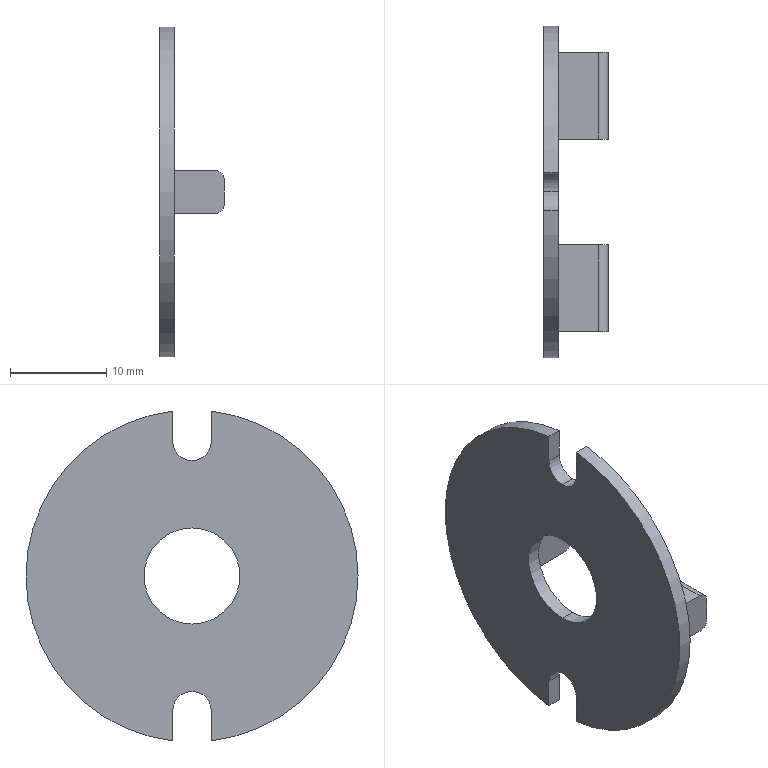Part | SolidWorks | features BaseBody 3 | 3 solids | 29 faces | box 6.7 x 34.5 x 34.267 mm | volume 1641 mm3 | plane 18 | cylinder 11 | commonest cylinder face diameters 2 x4 4 x3 10 x2 34.5 x2
STEP:
#1=CARTESIAN_POINT('',(-0.75,0.,12.));
#2=VERTEX_POINT('',#1);
#3=CARTESIAN_POINT('',(0.75,0.,12.));
#4=VERTEX_POINT('',#3);
#5=CARTESIAN_POINT('',(-0.75,0.,12.));
#6=DIRECTION('',(1.,0.,0.));
#7=VECTOR('',#6,1000.);
#8=LINE('',#5,#7);
#9=EDGE_CURVE('',#2,#4,#8,.T.);
#10=ORIENTED_EDGE('',*,*,#9,.F.);
#11=CARTESIAN_POINT('',(-0.75,-2.,14.));
#12=VERTEX_POINT('',#11);
#13=CARTESIAN_POINT('',(-0.75,0.,14.));
#14=DIRECTION('',(1.,0.,0.));
#15=DIRECTION('',(0.,0.,-1.));
#16=AXIS2_PLACEMENT_3D('',#13,#14,#15);
#17=CIRCLE('',#16,2.);
#18=EDGE_CURVE('',#12,#2,#17,.T.);
#19=ORIENTED_EDGE('',*,*,#18,.F.);
#20=CARTESIAN_POINT('',(0.75,-2.,14.));
#21=VERTEX_POINT('',#20);
#22=CARTESIAN_POINT('',(-0.75,-2.,14.));
#23=DIRECTION('',(1.,0.,0.));
#24=VECTOR('',#23,1000.);
#25=LINE('',#22,#24);
#26=EDGE_CURVE('',#12,#21,#25,.T.);
#27=ORIENTED_EDGE('',*,*,#26,.T.);
#28=CARTESIAN_POINT('',(0.75,0.,14.));
#29=DIRECTION('',(1.,0.,0.));
#30=DIRECTION('',(0.,0.,-1.));
#31=AXIS2_PLACEMENT_3D('',#28,#29,#30);
#32=CIRCLE('',#31,2.);
#33=EDGE_CURVE('',#21,#4,#32,.T.);
#34=ORIENTED_EDGE('',*,*,#33,.T.);
#35=EDGE_LOOP('',(#10,#19,#27,#34));
#36=FACE_OUTER_BOUND('',#35,.T.);
#37=CARTESIAN_POINT('',(-0.75,0.,14.));
#38=DIRECTION('',(1.,0.,0.));
#39=DIRECTION('',(0.,0.,-1.));
#40=AXIS2_PLACEMENT_3D('',#37,#38,#39);
#41=CYLINDRICAL_SURFACE('',#40,2.);
#42=ADVANCED_FACE('',(#36),#41,.F.);
#43=CARTESIAN_POINT('',(-0.75,2.,14.));
#44=VERTEX_POINT('',#43);
#45=CARTESIAN_POINT('',(-0.75,2.,17.134));
#46=VERTEX_POINT('',#45);
#47=CARTESIAN_POINT('',(-0.75,2.,14.));
#48=DIRECTION('',(0.,0.,1.));
#49=VECTOR('',#48,1000.);
#50=LINE('',#47,#49);
#51=EDGE_CURVE('',#44,#46,#50,.T.);
#52=ORIENTED_EDGE('',*,*,#51,.F.);
#53=CARTESIAN_POINT('',(0.75,2.,14.));
#54=VERTEX_POINT('',#53);
#55=CARTESIAN_POINT('',(-0.75,2.,14.));
#56=DIRECTION('',(1.,0.,0.));
#57=VECTOR('',#56,1000.);
#58=LINE('',#55,#57);
#59=EDGE_CURVE('',#44,#54,#58,.T.);
#60=ORIENTED_EDGE('',*,*,#59,.T.);
#61=CARTESIAN_POINT('',(0.75,2.,17.134));
#62=VERTEX_POINT('',#61);
#63=CARTESIAN_POINT('',(0.75,2.,14.));
#64=DIRECTION('',(0.,0.,1.));
#65=VECTOR('',#64,1000.);
#66=LINE('',#63,#65);
#67=EDGE_CURVE('',#54,#62,#66,.T.);
#68=ORIENTED_EDGE('',*,*,#67,.T.);
#69=CARTESIAN_POINT('',(0.75,2.,17.134));
#70=DIRECTION('',(1.,0.,0.));
#71=VECTOR('',#70,1000.);
#72=LINE('',#69,#71);
#73=EDGE_CURVE('',#46,#62,#72,.T.);
#74=ORIENTED_EDGE('',*,*,#73,.F.);
#75=EDGE_LOOP('',(#52,#60,#68,#74));
#76=FACE_OUTER_BOUND('',#75,.T.);
#77=CARTESIAN_POINT('',(-0.75,2.,14.));
#78=DIRECTION('',(0.,1.,0.));
#79=DIRECTION('',(0.,0.,-1.));
#80=AXIS2_PLACEMENT_3D('',#77,#78,#79);
#81=PLANE('',#80);
#82=ADVANCED_FACE('',(#76),#81,.F.);
#83=CARTESIAN_POINT('',(0.75,-2.,17.134));
#84=VERTEX_POINT('',#83);
#85=CARTESIAN_POINT('',(0.75,-2.,14.));
#86=DIRECTION('',(0.,0.,-1.));
#87=VECTOR('',#86,1000.);
#88=LINE('',#85,#87);
#89=EDGE_CURVE('',#84,#21,#88,.T.);
#90=ORIENTED_EDGE('',*,*,#89,.T.);
#91=ORIENTED_EDGE('',*,*,#26,.F.);
#92=CARTESIAN_POINT('',(-0.75,-2.,17.134));
#93=VERTEX_POINT('',#92);
#94=CARTESIAN_POINT('',(-0.75,-2.,14.));
#95=DIRECTION('',(0.,0.,-1.));
#96=VECTOR('',#95,1000.);
#97=LINE('',#94,#96);
#98=EDGE_CURVE('',#93,#12,#97,.T.);
#99=ORIENTED_EDGE('',*,*,#98,.F.);
#100=CARTESIAN_POINT('',(0.75,-2.,17.134));
#101=DIRECTION('',(-1.,0.,0.));
#102=VECTOR('',#101,1000.);
#103=LINE('',#100,#102);
#104=EDGE_CURVE('',#84,#93,#103,.T.);
#105=ORIENTED_EDGE('',*,*,#104,.F.);
#106=EDGE_LOOP('',(#90,#91,#99,#105));
#107=FACE_OUTER_BOUND('',#106,.T.);
#108=CARTESIAN_POINT('',(-0.75,-2.,14.));
#109=DIRECTION('',(0.,-1.,0.));
#110=DIRECTION('',(-1.,0.,0.));
#111=AXIS2_PLACEMENT_3D('',#108,#109,#110);
#112=PLANE('',#111);
#113=ADVANCED_FACE('',(#107),#112,.F.);
#114=CARTESIAN_POINT('',(0.75,2.,-14.));
#115=VERTEX_POINT('',#114);
#116=CARTESIAN_POINT('',(0.75,-2.,-14.));
#117=VERTEX_POINT('',#116);
#118=CARTESIAN_POINT('',(0.75,0.,-14.));
#119=DIRECTION('',(1.,0.,0.));
#120=DIRECTION('',(0.,0.,1.));
#121=AXIS2_PLACEMENT_3D('',#118,#119,#120);
#122=CIRCLE('',#121,2.);
#123=EDGE_CURVE('',#115,#117,#122,.T.);
#124=ORIENTED_EDGE('',*,*,#123,.T.);
#125=CARTESIAN_POINT('',(-0.75,-2.,-14.));
#126=VERTEX_POINT('',#125);
#127=CARTESIAN_POINT('',(-0.75,-2.,-14.));
#128=DIRECTION('',(1.,0.,0.));
#129=VECTOR('',#128,1000.);
#130=LINE('',#127,#129);
#131=EDGE_CURVE('',#126,#117,#130,.T.);
#132=ORIENTED_EDGE('',*,*,#131,.F.);
#133=CARTESIAN_POINT('',(-0.75,2.,-14.));
#134=VERTEX_POINT('',#133);
#135=CARTESIAN_POINT('',(-0.75,0.,-14.));
#136=DIRECTION('',(1.,0.,0.));
#137=DIRECTION('',(0.,0.,1.));
#138=AXIS2_PLACEMENT_3D('',#135,#136,#137);
#139=CIRCLE('',#138,2.);
#140=EDGE_CURVE('',#134,#126,#139,.T.);
#141=ORIENTED_EDGE('',*,*,#140,.F.);
#142=CARTESIAN_POINT('',(-0.75,2.,-14.));
#143=DIRECTION('',(1.,0.,0.));
#144=VECTOR('',#143,1000.);
#145=LINE('',#142,#144);
#146=EDGE_CURVE('',#134,#115,#145,.T.);
#147=ORIENTED_EDGE('',*,*,#146,.T.);
#148=EDGE_LOOP('',(#124,#132,#141,#147));
#149=FACE_OUTER_BOUND('',#148,.T.);
#150=CARTESIAN_POINT('',(-0.75,0.,-14.));
#151=DIRECTION('',(1.,0.,0.));
#152=DIRECTION('',(0.,0.,-1.));
#153=AXIS2_PLACEMENT_3D('',#150,#151,#152);
#154=CYLINDRICAL_SURFACE('',#153,2.);
#155=ADVANCED_FACE('',(#149),#154,.F.);
#156=CARTESIAN_POINT('',(-0.75,-2.,-17.134));
#157=VERTEX_POINT('',#156);
#158=CARTESIAN_POINT('',(-0.75,-2.,-14.));
#159=DIRECTION('',(0.,0.,-1.));
#160=VECTOR('',#159,1000.);
#161=LINE('',#158,#160);
#162=EDGE_CURVE('',#126,#157,#161,.T.);
#163=ORIENTED_EDGE('',*,*,#162,.F.);
#164=ORIENTED_EDGE('',*,*,#131,.T.);
#165=CARTESIAN_POINT('',(0.75,-2.,-17.134));
#166=VERTEX_POINT('',#165);
#167=CARTESIAN_POINT('',(0.75,-2.,-14.));
#168=DIRECTION('',(0.,0.,-1.));
#169=VECTOR('',#168,1000.);
#170=LINE('',#167,#169);
#171=EDGE_CURVE('',#117,#166,#170,.T.);
#172=ORIENTED_EDGE('',*,*,#171,.T.);
#173=CARTESIAN_POINT('',(0.75,-2.,-17.134));
#174=DIRECTION('',(1.,0.,0.));
#175=VECTOR('',#174,1000.);
#176=LINE('',#173,#175);
#177=EDGE_CURVE('',#157,#166,#176,.T.);
#178=ORIENTED_EDGE('',*,*,#177,.F.);
#179=EDGE_LOOP('',(#163,#164,#172,#178));
#180=FACE_OUTER_BOUND('',#179,.T.);
#181=CARTESIAN_POINT('',(-0.75,-2.,-14.));
#182=DIRECTION('',(0.,-1.,0.));
#183=DIRECTION('',(0.,0.,-1.));
#184=AXIS2_PLACEMENT_3D('',#181,#182,#183);
#185=PLANE('',#184);
#186=ADVANCED_FACE('',(#180),#185,.F.);
#187=CARTESIAN_POINT('',(0.75,2.,-17.134));
#188=VERTEX_POINT('',#187);
#189=CARTESIAN_POINT('',(0.75,2.,-14.));
#190=DIRECTION('',(0.,0.,1.));
#191=VECTOR('',#190,1000.);
#192=LINE('',#189,#191);
#193=EDGE_CURVE('',#188,#115,#192,.T.);
#194=ORIENTED_EDGE('',*,*,#193,.T.);
#195=ORIENTED_EDGE('',*,*,#146,.F.);
#196=CARTESIAN_POINT('',(-0.75,2.,-17.134));
#197=VERTEX_POINT('',#196);
#198=CARTESIAN_POINT('',(-0.75,2.,-14.));
#199=DIRECTION('',(0.,0.,1.));
#200=VECTOR('',#199,1000.);
#201=LINE('',#198,#200);
#202=EDGE_CURVE('',#197,#134,#201,.T.);
#203=ORIENTED_EDGE('',*,*,#202,.F.);
#204=CARTESIAN_POINT('',(0.75,2.,-17.134));
#205=DIRECTION('',(-1.,0.,0.));
#206=VECTOR('',#205,1000.);
#207=LINE('',#204,#206);
#208=EDGE_CURVE('',#188,#197,#207,.T.);
#209=ORIENTED_EDGE('',*,*,#208,.F.);
#210=EDGE_LOOP('',(#194,#195,#203,#209));
#211=FACE_OUTER_BOUND('',#210,.T.);
#212=CARTESIAN_POINT('',(-0.75,2.,-14.));
#213=DIRECTION('',(0.,1.,0.));
#214=DIRECTION('',(0.,0.,-1.));
#215=AXIS2_PLACEMENT_3D('',#212,#213,#214);
#216=PLANE('',#215);
#217=ADVANCED_FACE('',(#211),#216,.F.);
#218=CARTESIAN_POINT('',(0.75,0.,-5.));
#219=VERTEX_POINT('',#218);
#220=CARTESIAN_POINT('',(-0.75,0.,-5.));
#221=VERTEX_POINT('',#220);
#222=CARTESIAN_POINT('',(0.75,0.,-5.));
#223=DIRECTION('',(-1.,0.,0.));
#224=VECTOR('',#223,1000.);
#225=LINE('',#222,#224);
#226=EDGE_CURVE('',#219,#221,#225,.T.);
#227=ORIENTED_EDGE('',*,*,#226,.F.);
#228=CARTESIAN_POINT('',(0.75,0.,5.));
#229=VERTEX_POINT('',#228);
#230=CARTESIAN_POINT('',(0.75,0.,0.));
#231=DIRECTION('',(1.,0.,0.));
#232=DIRECTION('',(0.,0.,-1.));
#233=AXIS2_PLACEMENT_3D('',#230,#231,#232);
#234=CIRCLE('',#233,5.);
#235=EDGE_CURVE('',#219,#229,#234,.T.);
#236=ORIENTED_EDGE('',*,*,#235,.T.);
#237=CARTESIAN_POINT('',(-0.75,0.,5.));
#238=VERTEX_POINT('',#237);
#239=CARTESIAN_POINT('',(0.75,0.,5.));
#240=DIRECTION('',(-1.,0.,0.));
#241=VECTOR('',#240,1000.);
#242=LINE('',#239,#241);
#243=EDGE_CURVE('',#229,#238,#242,.T.);
#244=ORIENTED_EDGE('',*,*,#243,.T.);
#245=CARTESIAN_POINT('',(-0.75,0.,0.));
#246=DIRECTION('',(1.,0.,0.));
#247=DIRECTION('',(0.,0.,-1.));
#248=AXIS2_PLACEMENT_3D('',#245,#246,#247);
#249=CIRCLE('',#248,5.);
#250=EDGE_CURVE('',#221,#238,#249,.T.);
#251=ORIENTED_EDGE('',*,*,#250,.F.);
#252=EDGE_LOOP('',(#227,#236,#244,#251));
#253=FACE_OUTER_BOUND('',#252,.T.);
#254=CARTESIAN_POINT('',(0.75,0.,0.));
#255=DIRECTION('',(-1.,0.,0.));
#256=DIRECTION('',(0.,0.,1.));
#257=AXIS2_PLACEMENT_3D('',#254,#255,#256);
#258=CYLINDRICAL_SURFACE('',#257,5.);
#259=ADVANCED_FACE('',(#253),#258,.F.);
#260=CARTESIAN_POINT('',(-0.75,0.,0.));
#261=DIRECTION('',(1.,0.,0.));
#262=DIRECTION('',(0.,0.,-1.));
#263=AXIS2_PLACEMENT_3D('',#260,#261,#262);
#264=CIRCLE('',#263,17.25);
#265=EDGE_CURVE('',#197,#46,#264,.T.);
#266=ORIENTED_EDGE('',*,*,#265,.T.);
#267=ORIENTED_EDGE('',*,*,#73,.T.);
#268=CARTESIAN_POINT('',(0.75,0.,0.));
#269=DIRECTION('',(1.,0.,0.));
#270=DIRECTION('',(0.,0.,-1.));
#271=AXIS2_PLACEMENT_3D('',#268,#269,#270);
#272=CIRCLE('',#271,17.25);
#273=EDGE_CURVE('',#188,#62,#272,.T.);
#274=ORIENTED_EDGE('',*,*,#273,.F.);
#275=ORIENTED_EDGE('',*,*,#208,.T.);
#276=EDGE_LOOP('',(#266,#267,#274,#275));
#277=FACE_OUTER_BOUND('',#276,.T.);
#278=CARTESIAN_POINT('',(0.75,0.,0.));
#279=DIRECTION('',(-1.,0.,0.));
#280=DIRECTION('',(0.,0.,1.));
#281=AXIS2_PLACEMENT_3D('',#278,#279,#280);
#282=CYLINDRICAL_SURFACE('',#281,17.25);
#283=ADVANCED_FACE('',(#277),#282,.T.);
#284=CARTESIAN_POINT('',(-0.75,0.,0.));
#285=DIRECTION('',(1.,0.,0.));
#286=DIRECTION('',(0.,0.,-1.));
#287=AXIS2_PLACEMENT_3D('',#284,#285,#286);
#288=CIRCLE('',#287,5.);
#289=EDGE_CURVE('',#238,#221,#288,.T.);
#290=ORIENTED_EDGE('',*,*,#289,.T.);
#291=ORIENTED_EDGE('',*,*,#250,.T.);
#292=EDGE_LOOP('',(#290,#291));
#293=FACE_BOUND('',#292,.T.);
#294=CARTESIAN_POINT('',(-0.75,0.,0.));
#295=DIRECTION('',(1.,0.,0.));
#296=DIRECTION('',(0.,0.,-1.));
#297=AXIS2_PLACEMENT_3D('',#294,#295,#296);
#298=CIRCLE('',#297,17.25);
#299=EDGE_CURVE('',#93,#157,#298,.T.);
#300=ORIENTED_EDGE('',*,*,#299,.F.);
#301=ORIENTED_EDGE('',*,*,#98,.T.);
#302=ORIENTED_EDGE('',*,*,#18,.T.);
#303=CARTESIAN_POINT('',(-0.75,0.,14.));
#304=DIRECTION('',(1.,0.,0.));
#305=DIRECTION('',(0.,0.,-1.));
#306=AXIS2_PLACEMENT_3D('',#303,#304,#305);
#307=CIRCLE('',#306,2.);
#308=EDGE_CURVE('',#2,#44,#307,.T.);
#309=ORIENTED_EDGE('',*,*,#308,.T.);
#310=ORIENTED_EDGE('',*,*,#51,.T.);
#311=ORIENTED_EDGE('',*,*,#265,.F.);
#312=ORIENTED_EDGE('',*,*,#202,.T.);
#313=ORIENTED_EDGE('',*,*,#140,.T.);
#314=ORIENTED_EDGE('',*,*,#162,.T.);
#315=EDGE_LOOP('',(#300,#301,#302,#309,#310,#311,#312,#313,#314));
#316=FACE_OUTER_BOUND('',#315,.T.);
#317=CARTESIAN_POINT('',(-0.75,0.,0.));
#318=DIRECTION('',(1.,0.,0.));
#319=DIRECTION('',(0.,1.,0.));
#320=AXIS2_PLACEMENT_3D('',#317,#318,#319);
#321=PLANE('',#320);
#322=ADVANCED_FACE('',(#293,#316),#321,.F.);
#323=CARTESIAN_POINT('',(0.75,0.,0.));
#324=DIRECTION('',(1.,0.,0.));
#325=DIRECTION('',(0.,0.,-1.));
#326=AXIS2_PLACEMENT_3D('',#323,#324,#325);
#327=CIRCLE('',#326,5.);
#328=EDGE_CURVE('',#229,#219,#327,.T.);
#329=ORIENTED_EDGE('',*,*,#328,.F.);
#330=ORIENTED_EDGE('',*,*,#235,.F.);
#331=EDGE_LOOP('',(#329,#330));
#332=FACE_BOUND('',#331,.T.);
#333=ORIENTED_EDGE('',*,*,#89,.F.);
#334=CARTESIAN_POINT('',(0.75,0.,0.));
#335=DIRECTION('',(1.,0.,0.));
#336=DIRECTION('',(0.,0.,-1.));
#337=AXIS2_PLACEMENT_3D('',#334,#335,#336);
#338=CIRCLE('',#337,17.25);
#339=EDGE_CURVE('',#84,#166,#338,.T.);
#340=ORIENTED_EDGE('',*,*,#339,.T.);
#341=ORIENTED_EDGE('',*,*,#171,.F.);
#342=ORIENTED_EDGE('',*,*,#123,.F.);
#343=ORIENTED_EDGE('',*,*,#193,.F.);
#344=ORIENTED_EDGE('',*,*,#273,.T.);
#345=ORIENTED_EDGE('',*,*,#67,.F.);
#346=CARTESIAN_POINT('',(0.75,0.,14.));
#347=DIRECTION('',(1.,0.,0.));
#348=DIRECTION('',(0.,0.,-1.));
#349=AXIS2_PLACEMENT_3D('',#346,#347,#348);
#350=CIRCLE('',#349,2.);
#351=EDGE_CURVE('',#4,#54,#350,.T.);
#352=ORIENTED_EDGE('',*,*,#351,.F.);
#353=ORIENTED_EDGE('',*,*,#33,.F.);
#354=EDGE_LOOP('',(#333,#340,#341,#342,#343,#344,#345,#352,#353));
#355=FACE_OUTER_BOUND('',#354,.T.);
#356=CARTESIAN_POINT('',(0.75,0.,0.));
#357=DIRECTION('',(1.,0.,0.));
#358=DIRECTION('',(0.,1.,0.));
#359=AXIS2_PLACEMENT_3D('',#356,#357,#358);
#360=PLANE('',#359);
#361=ADVANCED_FACE('',(#332,#355),#360,.T.);
#362=ORIENTED_EDGE('',*,*,#339,.F.);
#363=ORIENTED_EDGE('',*,*,#104,.T.);
#364=ORIENTED_EDGE('',*,*,#299,.T.);
#365=ORIENTED_EDGE('',*,*,#177,.T.);
#366=EDGE_LOOP('',(#362,#363,#364,#365));
#367=FACE_OUTER_BOUND('',#366,.T.);
#368=CARTESIAN_POINT('',(0.75,0.,0.));
#369=DIRECTION('',(-1.,0.,0.));
#370=DIRECTION('',(0.,0.,1.));
#371=AXIS2_PLACEMENT_3D('',#368,#369,#370);
#372=CYLINDRICAL_SURFACE('',#371,17.25);
#373=ADVANCED_FACE('',(#367),#372,.T.);
#374=ORIENTED_EDGE('',*,*,#328,.T.);
#375=ORIENTED_EDGE('',*,*,#226,.T.);
#376=ORIENTED_EDGE('',*,*,#289,.F.);
#377=ORIENTED_EDGE('',*,*,#243,.F.);
#378=EDGE_LOOP('',(#374,#375,#376,#377));
#379=FACE_OUTER_BOUND('',#378,.T.);
#380=CARTESIAN_POINT('',(0.75,0.,0.));
#381=DIRECTION('',(-1.,0.,0.));
#382=DIRECTION('',(0.,0.,1.));
#383=AXIS2_PLACEMENT_3D('',#380,#381,#382);
#384=CYLINDRICAL_SURFACE('',#383,5.);
#385=ADVANCED_FACE('',(#379),#384,.F.);
#386=ORIENTED_EDGE('',*,*,#308,.F.);
#387=ORIENTED_EDGE('',*,*,#9,.T.);
#388=ORIENTED_EDGE('',*,*,#351,.T.);
#389=ORIENTED_EDGE('',*,*,#59,.F.);
#390=EDGE_LOOP('',(#386,#387,#388,#389));
#391=FACE_OUTER_BOUND('',#390,.T.);
#392=CARTESIAN_POINT('',(-0.75,0.,14.));
#393=DIRECTION('',(1.,0.,0.));
#394=DIRECTION('',(0.,0.,-1.));
#395=AXIS2_PLACEMENT_3D('',#392,#393,#394);
#396=CYLINDRICAL_SURFACE('',#395,2.);
#397=ADVANCED_FACE('',(#391),#396,.F.);
#398=CLOSED_SHELL('',(#42,#82,#113,#155,#186,#217,#259,#283,#322,#361,#373,#385,#397));
#399=MANIFOLD_SOLID_BREP('',#398);
#400=CARTESIAN_POINT('',(4.95,14.5,2.25));
#401=VERTEX_POINT('',#400);
#402=CARTESIAN_POINT('',(5.95,14.5,1.25));
#403=VERTEX_POINT('',#402);
#404=CARTESIAN_POINT('',(4.95,14.5,1.25));
#405=DIRECTION('',(0.,1.,0.));
#406=DIRECTION('',(0.,0.,-1.));
#407=AXIS2_PLACEMENT_3D('',#404,#405,#406);
#408=CIRCLE('',#407,1.);
#409=EDGE_CURVE('',#401,#403,#408,.T.);
#410=ORIENTED_EDGE('',*,*,#409,.F.);
#411=CARTESIAN_POINT('',(4.95,5.5,2.25));
#412=VERTEX_POINT('',#411);
#413=CARTESIAN_POINT('',(4.95,5.5,2.25));
#414=DIRECTION('',(0.,1.,0.));
#415=VECTOR('',#414,1000.);
#416=LINE('',#413,#415);
#417=EDGE_CURVE('',#412,#401,#416,.T.);
#418=ORIENTED_EDGE('',*,*,#417,.F.);
#419=CARTESIAN_POINT('',(5.95,5.5,1.25));
#420=VERTEX_POINT('',#419);
#421=CARTESIAN_POINT('',(4.95,5.5,1.25));
#422=DIRECTION('',(0.,-1.,0.));
#423=DIRECTION('',(0.,0.,1.));
#424=AXIS2_PLACEMENT_3D('',#421,#422,#423);
#425=CIRCLE('',#424,1.);
#426=EDGE_CURVE('',#420,#412,#425,.T.);
#427=ORIENTED_EDGE('',*,*,#426,.F.);
#428=CARTESIAN_POINT('',(5.95,0.,1.25));
#429=DIRECTION('',(0.,-1.,0.));
#430=VECTOR('',#429,1000.);
#431=LINE('',#428,#430);
#432=EDGE_CURVE('',#403,#420,#431,.T.);
#433=ORIENTED_EDGE('',*,*,#432,.F.);
#434=EDGE_LOOP('',(#410,#418,#427,#433));
#435=FACE_OUTER_BOUND('',#434,.T.);
#436=CARTESIAN_POINT('',(4.95,0.,1.25));
#437=DIRECTION('',(0.,-1.,0.));
#438=DIRECTION('',(0.,0.,-1.));
#439=AXIS2_PLACEMENT_3D('',#436,#437,#438);
#440=CYLINDRICAL_SURFACE('',#439,1.);
#441=ADVANCED_FACE('',(#435),#440,.T.);
#442=CARTESIAN_POINT('',(4.95,5.5,-2.25));
#443=VERTEX_POINT('',#442);
#444=CARTESIAN_POINT('',(5.95,5.5,-1.25));
#445=VERTEX_POINT('',#444);
#446=CARTESIAN_POINT('',(4.95,5.5,-1.25));
#447=DIRECTION('',(0.,-1.,0.));
#448=DIRECTION('',(0.,0.,1.));
#449=AXIS2_PLACEMENT_3D('',#446,#447,#448);
#450=CIRCLE('',#449,1.);
#451=EDGE_CURVE('',#443,#445,#450,.T.);
#452=ORIENTED_EDGE('',*,*,#451,.F.);
#453=CARTESIAN_POINT('',(4.95,14.5,-2.25));
#454=VERTEX_POINT('',#453);
#455=CARTESIAN_POINT('',(4.95,5.5,-2.25));
#456=DIRECTION('',(0.,-1.,0.));
#457=VECTOR('',#456,1000.);
#458=LINE('',#455,#457);
#459=EDGE_CURVE('',#454,#443,#458,.T.);
#460=ORIENTED_EDGE('',*,*,#459,.F.);
#461=CARTESIAN_POINT('',(5.95,14.5,-1.25));
#462=VERTEX_POINT('',#461);
#463=CARTESIAN_POINT('',(4.95,14.5,-1.25));
#464=DIRECTION('',(0.,1.,0.));
#465=DIRECTION('',(0.,0.,-1.));
#466=AXIS2_PLACEMENT_3D('',#463,#464,#465);
#467=CIRCLE('',#466,1.);
#468=EDGE_CURVE('',#462,#454,#467,.T.);
#469=ORIENTED_EDGE('',*,*,#468,.F.);
#470=CARTESIAN_POINT('',(5.95,0.,-1.25));
#471=DIRECTION('',(0.,1.,0.));
#472=VECTOR('',#471,1000.);
#473=LINE('',#470,#472);
#474=EDGE_CURVE('',#445,#462,#473,.T.);
#475=ORIENTED_EDGE('',*,*,#474,.F.);
#476=EDGE_LOOP('',(#452,#460,#469,#475));
#477=FACE_OUTER_BOUND('',#476,.T.);
#478=CARTESIAN_POINT('',(4.95,0.,-1.25));
#479=DIRECTION('',(0.,1.,0.));
#480=DIRECTION('',(0.,0.,1.));
#481=AXIS2_PLACEMENT_3D('',#478,#479,#480);
#482=CYLINDRICAL_SURFACE('',#481,1.);
#483=ADVANCED_FACE('',(#477),#482,.T.);
#484=CARTESIAN_POINT('',(0.75,5.5,-2.25));
#485=VERTEX_POINT('',#484);
#486=CARTESIAN_POINT('',(0.75,14.5,-2.25));
#487=VERTEX_POINT('',#486);
#488=CARTESIAN_POINT('',(0.75,5.5,-2.25));
#489=DIRECTION('',(0.,1.,0.));
#490=VECTOR('',#489,1000.);
#491=LINE('',#488,#490);
#492=EDGE_CURVE('',#485,#487,#491,.T.);
#493=ORIENTED_EDGE('',*,*,#492,.F.);
#494=CARTESIAN_POINT('',(0.75,5.5,2.25));
#495=VERTEX_POINT('',#494);
#496=CARTESIAN_POINT('',(0.75,5.5,2.25));
#497=DIRECTION('',(0.,0.,-1.));
#498=VECTOR('',#497,1000.);
#499=LINE('',#496,#498);
#500=EDGE_CURVE('',#495,#485,#499,.T.);
#501=ORIENTED_EDGE('',*,*,#500,.F.);
#502=CARTESIAN_POINT('',(0.75,14.5,2.25));
#503=VERTEX_POINT('',#502);
#504=CARTESIAN_POINT('',(0.75,5.5,2.25));
#505=DIRECTION('',(0.,-1.,0.));
#506=VECTOR('',#505,1000.);
#507=LINE('',#504,#506);
#508=EDGE_CURVE('',#503,#495,#507,.T.);
#509=ORIENTED_EDGE('',*,*,#508,.F.);
#510=CARTESIAN_POINT('',(0.75,14.5,2.25));
#511=DIRECTION('',(0.,0.,1.));
#512=VECTOR('',#511,1000.);
#513=LINE('',#510,#512);
#514=EDGE_CURVE('',#487,#503,#513,.T.);
#515=ORIENTED_EDGE('',*,*,#514,.F.);
#516=EDGE_LOOP('',(#493,#501,#509,#515));
#517=FACE_OUTER_BOUND('',#516,.T.);
#518=CARTESIAN_POINT('',(0.75,0.,0.));
#519=DIRECTION('',(-1.,0.,0.));
#520=DIRECTION('',(0.,0.,1.));
#521=AXIS2_PLACEMENT_3D('',#518,#519,#520);
#522=PLANE('',#521);
#523=ADVANCED_FACE('',(#517),#522,.T.);
#524=CARTESIAN_POINT('',(5.95,5.5,2.25));
#525=DIRECTION('',(0.,0.,-1.));
#526=VECTOR('',#525,1000.);
#527=LINE('',#524,#526);
#528=EDGE_CURVE('',#420,#445,#527,.T.);
#529=ORIENTED_EDGE('',*,*,#528,.T.);
#530=ORIENTED_EDGE('',*,*,#474,.T.);
#531=CARTESIAN_POINT('',(5.95,14.5,2.25));
#532=DIRECTION('',(0.,0.,1.));
#533=VECTOR('',#532,1000.);
#534=LINE('',#531,#533);
#535=EDGE_CURVE('',#462,#403,#534,.T.);
#536=ORIENTED_EDGE('',*,*,#535,.T.);
#537=ORIENTED_EDGE('',*,*,#432,.T.);
#538=EDGE_LOOP('',(#529,#530,#536,#537));
#539=FACE_OUTER_BOUND('',#538,.T.);
#540=CARTESIAN_POINT('',(5.95,0.,0.));
#541=DIRECTION('',(-1.,0.,0.));
#542=DIRECTION('',(0.,0.,1.));
#543=AXIS2_PLACEMENT_3D('',#540,#541,#542);
#544=PLANE('',#543);
#545=ADVANCED_FACE('',(#539),#544,.F.);
#546=CARTESIAN_POINT('',(5.95,5.5,-2.25));
#547=DIRECTION('',(-1.,0.,0.));
#548=VECTOR('',#547,1000.);
#549=LINE('',#546,#548);
#550=EDGE_CURVE('',#443,#485,#549,.T.);
#551=ORIENTED_EDGE('',*,*,#550,.F.);
#552=ORIENTED_EDGE('',*,*,#451,.T.);
#553=ORIENTED_EDGE('',*,*,#528,.F.);
#554=ORIENTED_EDGE('',*,*,#426,.T.);
#555=CARTESIAN_POINT('',(5.95,5.5,2.25));
#556=DIRECTION('',(-1.,0.,0.));
#557=VECTOR('',#556,1000.);
#558=LINE('',#555,#557);
#559=EDGE_CURVE('',#412,#495,#558,.T.);
#560=ORIENTED_EDGE('',*,*,#559,.T.);
#561=ORIENTED_EDGE('',*,*,#500,.T.);
#562=EDGE_LOOP('',(#551,#552,#553,#554,#560,#561));
#563=FACE_OUTER_BOUND('',#562,.T.);
#564=CARTESIAN_POINT('',(5.95,5.5,2.25));
#565=DIRECTION('',(0.,1.,0.));
#566=DIRECTION('',(1.,0.,0.));
#567=AXIS2_PLACEMENT_3D('',#564,#565,#566);
#568=PLANE('',#567);
#569=ADVANCED_FACE('',(#563),#568,.F.);
#570=ORIENTED_EDGE('',*,*,#559,.F.);
#571=ORIENTED_EDGE('',*,*,#417,.T.);
#572=CARTESIAN_POINT('',(5.95,14.5,2.25));
#573=DIRECTION('',(-1.,0.,0.));
#574=VECTOR('',#573,1000.);
#575=LINE('',#572,#574);
#576=EDGE_CURVE('',#401,#503,#575,.T.);
#577=ORIENTED_EDGE('',*,*,#576,.T.);
#578=ORIENTED_EDGE('',*,*,#508,.T.);
#579=EDGE_LOOP('',(#570,#571,#577,#578));
#580=FACE_OUTER_BOUND('',#579,.T.);
#581=CARTESIAN_POINT('',(5.95,5.5,2.25));
#582=DIRECTION('',(0.,0.,-1.));
#583=DIRECTION('',(-1.,0.,0.));
#584=AXIS2_PLACEMENT_3D('',#581,#582,#583);
#585=PLANE('',#584);
#586=ADVANCED_FACE('',(#580),#585,.F.);
#587=ORIENTED_EDGE('',*,*,#535,.F.);
#588=ORIENTED_EDGE('',*,*,#468,.T.);
#589=CARTESIAN_POINT('',(5.95,14.5,-2.25));
#590=DIRECTION('',(-1.,0.,0.));
#591=VECTOR('',#590,1000.);
#592=LINE('',#589,#591);
#593=EDGE_CURVE('',#454,#487,#592,.T.);
#594=ORIENTED_EDGE('',*,*,#593,.T.);
#595=ORIENTED_EDGE('',*,*,#514,.T.);
#596=ORIENTED_EDGE('',*,*,#576,.F.);
#597=ORIENTED_EDGE('',*,*,#409,.T.);
#598=EDGE_LOOP('',(#587,#588,#594,#595,#596,#597));
#599=FACE_OUTER_BOUND('',#598,.T.);
#600=CARTESIAN_POINT('',(5.95,14.5,2.25));
#601=DIRECTION('',(0.,-1.,0.));
#602=DIRECTION('',(0.,0.,-1.));
#603=AXIS2_PLACEMENT_3D('',#600,#601,#602);
#604=PLANE('',#603);
#605=ADVANCED_FACE('',(#599),#604,.F.);
#606=ORIENTED_EDGE('',*,*,#593,.F.);
#607=ORIENTED_EDGE('',*,*,#459,.T.);
#608=ORIENTED_EDGE('',*,*,#550,.T.);
#609=ORIENTED_EDGE('',*,*,#492,.T.);
#610=EDGE_LOOP('',(#606,#607,#608,#609));
#611=FACE_OUTER_BOUND('',#610,.T.);
#612=CARTESIAN_POINT('',(5.95,5.5,-2.25));
#613=DIRECTION('',(0.,0.,1.));
#614=DIRECTION('',(0.,-1.,0.));
#615=AXIS2_PLACEMENT_3D('',#612,#613,#614);
#616=PLANE('',#615);
#617=ADVANCED_FACE('',(#611),#616,.F.);
#618=CLOSED_SHELL('',(#441,#483,#523,#545,#569,#586,#605,#617));
#619=MANIFOLD_SOLID_BREP('',#618);
#620=CARTESIAN_POINT('',(4.95,-5.5,2.25));
#621=VERTEX_POINT('',#620);
#622=CARTESIAN_POINT('',(5.95,-5.5,1.25));
#623=VERTEX_POINT('',#622);
#624=CARTESIAN_POINT('',(4.95,-5.5,1.25));
#625=DIRECTION('',(0.,1.,0.));
#626=DIRECTION('',(0.,0.,-1.));
#627=AXIS2_PLACEMENT_3D('',#624,#625,#626);
#628=CIRCLE('',#627,1.);
#629=EDGE_CURVE('',#621,#623,#628,.T.);
#630=ORIENTED_EDGE('',*,*,#629,.F.);
#631=CARTESIAN_POINT('',(4.95,-14.5,2.25));
#632=VERTEX_POINT('',#631);
#633=CARTESIAN_POINT('',(4.95,-5.5,2.25));
#634=DIRECTION('',(0.,1.,0.));
#635=VECTOR('',#634,1000.);
#636=LINE('',#633,#635);
#637=EDGE_CURVE('',#632,#621,#636,.T.);
#638=ORIENTED_EDGE('',*,*,#637,.F.);
#639=CARTESIAN_POINT('',(5.95,-14.5,1.25));
#640=VERTEX_POINT('',#639);
#641=CARTESIAN_POINT('',(4.95,-14.5,1.25));
#642=DIRECTION('',(0.,-1.,0.));
#643=DIRECTION('',(0.,0.,1.));
#644=AXIS2_PLACEMENT_3D('',#641,#642,#643);
#645=CIRCLE('',#644,1.);
#646=EDGE_CURVE('',#640,#632,#645,.T.);
#647=ORIENTED_EDGE('',*,*,#646,.F.);
#648=CARTESIAN_POINT('',(5.95,-14.5,1.25));
#649=DIRECTION('',(0.,-1.,0.));
#650=VECTOR('',#649,1000.);
#651=LINE('',#648,#650);
#652=EDGE_CURVE('',#623,#640,#651,.T.);
#653=ORIENTED_EDGE('',*,*,#652,.F.);
#654=EDGE_LOOP('',(#630,#638,#647,#653));
#655=FACE_OUTER_BOUND('',#654,.T.);
#656=CARTESIAN_POINT('',(4.95,0.,1.25));
#657=DIRECTION('',(0.,1.,0.));
#658=DIRECTION('',(0.,0.,1.));
#659=AXIS2_PLACEMENT_3D('',#656,#657,#658);
#660=CYLINDRICAL_SURFACE('',#659,1.);
#661=ADVANCED_FACE('',(#655),#660,.T.);
#662=CARTESIAN_POINT('',(4.95,-14.5,-2.25));
#663=VERTEX_POINT('',#662);
#664=CARTESIAN_POINT('',(5.95,-14.5,-1.25));
#665=VERTEX_POINT('',#664);
#666=CARTESIAN_POINT('',(4.95,-14.5,-1.25));
#667=DIRECTION('',(0.,-1.,0.));
#668=DIRECTION('',(0.,0.,1.));
#669=AXIS2_PLACEMENT_3D('',#666,#667,#668);
#670=CIRCLE('',#669,1.);
#671=EDGE_CURVE('',#663,#665,#670,.T.);
#672=ORIENTED_EDGE('',*,*,#671,.F.);
#673=CARTESIAN_POINT('',(4.95,-5.5,-2.25));
#674=VERTEX_POINT('',#673);
#675=CARTESIAN_POINT('',(4.95,-14.5,-2.25));
#676=DIRECTION('',(0.,-1.,0.));
#677=VECTOR('',#676,1000.);
#678=LINE('',#675,#677);
#679=EDGE_CURVE('',#674,#663,#678,.T.);
#680=ORIENTED_EDGE('',*,*,#679,.F.);
#681=CARTESIAN_POINT('',(5.95,-5.5,-1.25));
#682=VERTEX_POINT('',#681);
#683=CARTESIAN_POINT('',(4.95,-5.5,-1.25));
#684=DIRECTION('',(0.,1.,0.));
#685=DIRECTION('',(0.,0.,-1.));
#686=AXIS2_PLACEMENT_3D('',#683,#684,#685);
#687=CIRCLE('',#686,1.);
#688=EDGE_CURVE('',#682,#674,#687,.T.);
#689=ORIENTED_EDGE('',*,*,#688,.F.);
#690=CARTESIAN_POINT('',(5.95,-5.5,-1.25));
#691=DIRECTION('',(0.,1.,0.));
#692=VECTOR('',#691,1000.);
#693=LINE('',#690,#692);
#694=EDGE_CURVE('',#665,#682,#693,.T.);
#695=ORIENTED_EDGE('',*,*,#694,.F.);
#696=EDGE_LOOP('',(#672,#680,#689,#695));
#697=FACE_OUTER_BOUND('',#696,.T.);
#698=CARTESIAN_POINT('',(4.95,0.,-1.25));
#699=DIRECTION('',(0.,-1.,0.));
#700=DIRECTION('',(0.,0.,-1.));
#701=AXIS2_PLACEMENT_3D('',#698,#699,#700);
#702=CYLINDRICAL_SURFACE('',#701,1.);
#703=ADVANCED_FACE('',(#697),#702,.T.);
#704=CARTESIAN_POINT('',(0.75,-5.5,2.25));
#705=VERTEX_POINT('',#704);
#706=CARTESIAN_POINT('',(0.75,-14.5,2.25));
#707=VERTEX_POINT('',#706);
#708=CARTESIAN_POINT('',(0.75,-5.5,2.25));
#709=DIRECTION('',(0.,-1.,0.));
#710=VECTOR('',#709,1000.);
#711=LINE('',#708,#710);
#712=EDGE_CURVE('',#705,#707,#711,.T.);
#713=ORIENTED_EDGE('',*,*,#712,.F.);
#714=CARTESIAN_POINT('',(0.75,-5.5,-2.25));
#715=VERTEX_POINT('',#714);
#716=CARTESIAN_POINT('',(0.75,-5.5,2.25));
#717=DIRECTION('',(0.,0.,1.));
#718=VECTOR('',#717,1000.);
#719=LINE('',#716,#718);
#720=EDGE_CURVE('',#715,#705,#719,.T.);
#721=ORIENTED_EDGE('',*,*,#720,.F.);
#722=CARTESIAN_POINT('',(0.75,-14.5,-2.25));
#723=VERTEX_POINT('',#722);
#724=CARTESIAN_POINT('',(0.75,-5.5,-2.25));
#725=DIRECTION('',(0.,1.,0.));
#726=VECTOR('',#725,1000.);
#727=LINE('',#724,#726);
#728=EDGE_CURVE('',#723,#715,#727,.T.);
#729=ORIENTED_EDGE('',*,*,#728,.F.);
#730=CARTESIAN_POINT('',(0.75,-14.5,2.25));
#731=DIRECTION('',(0.,0.,-1.));
#732=VECTOR('',#731,1000.);
#733=LINE('',#730,#732);
#734=EDGE_CURVE('',#707,#723,#733,.T.);
#735=ORIENTED_EDGE('',*,*,#734,.F.);
#736=EDGE_LOOP('',(#713,#721,#729,#735));
#737=FACE_OUTER_BOUND('',#736,.T.);
#738=CARTESIAN_POINT('',(0.75,0.,0.));
#739=DIRECTION('',(1.,0.,0.));
#740=DIRECTION('',(0.,1.,0.));
#741=AXIS2_PLACEMENT_3D('',#738,#739,#740);
#742=PLANE('',#741);
#743=ADVANCED_FACE('',(#737),#742,.F.);
#744=CARTESIAN_POINT('',(5.95,-14.5,2.25));
#745=DIRECTION('',(0.,0.,-1.));
#746=VECTOR('',#745,1000.);
#747=LINE('',#744,#746);
#748=EDGE_CURVE('',#640,#665,#747,.T.);
#749=ORIENTED_EDGE('',*,*,#748,.T.);
#750=ORIENTED_EDGE('',*,*,#694,.T.);
#751=CARTESIAN_POINT('',(5.95,-5.5,2.25));
#752=DIRECTION('',(0.,0.,1.));
#753=VECTOR('',#752,1000.);
#754=LINE('',#751,#753);
#755=EDGE_CURVE('',#682,#623,#754,.T.);
#756=ORIENTED_EDGE('',*,*,#755,.T.);
#757=ORIENTED_EDGE('',*,*,#652,.T.);
#758=EDGE_LOOP('',(#749,#750,#756,#757));
#759=FACE_OUTER_BOUND('',#758,.T.);
#760=CARTESIAN_POINT('',(5.95,0.,0.));
#761=DIRECTION('',(1.,0.,0.));
#762=DIRECTION('',(0.,1.,0.));
#763=AXIS2_PLACEMENT_3D('',#760,#761,#762);
#764=PLANE('',#763);
#765=ADVANCED_FACE('',(#759),#764,.T.);
#766=ORIENTED_EDGE('',*,*,#755,.F.);
#767=ORIENTED_EDGE('',*,*,#688,.T.);
#768=CARTESIAN_POINT('',(5.95,-5.5,-2.25));
#769=DIRECTION('',(-1.,0.,0.));
#770=VECTOR('',#769,1000.);
#771=LINE('',#768,#770);
#772=EDGE_CURVE('',#674,#715,#771,.T.);
#773=ORIENTED_EDGE('',*,*,#772,.T.);
#774=ORIENTED_EDGE('',*,*,#720,.T.);
#775=CARTESIAN_POINT('',(5.95,-5.5,2.25));
#776=DIRECTION('',(-1.,0.,0.));
#777=VECTOR('',#776,1000.);
#778=LINE('',#775,#777);
#779=EDGE_CURVE('',#621,#705,#778,.T.);
#780=ORIENTED_EDGE('',*,*,#779,.F.);
#781=ORIENTED_EDGE('',*,*,#629,.T.);
#782=EDGE_LOOP('',(#766,#767,#773,#774,#780,#781));
#783=FACE_OUTER_BOUND('',#782,.T.);
#784=CARTESIAN_POINT('',(5.95,-5.5,2.25));
#785=DIRECTION('',(0.,-1.,0.));
#786=DIRECTION('',(0.,0.,-1.));
#787=AXIS2_PLACEMENT_3D('',#784,#785,#786);
#788=PLANE('',#787);
#789=ADVANCED_FACE('',(#783),#788,.F.);
#790=ORIENTED_EDGE('',*,*,#772,.F.);
#791=ORIENTED_EDGE('',*,*,#679,.T.);
#792=CARTESIAN_POINT('',(5.95,-14.5,-2.25));
#793=DIRECTION('',(-1.,0.,0.));
#794=VECTOR('',#793,1000.);
#795=LINE('',#792,#794);
#796=EDGE_CURVE('',#663,#723,#795,.T.);
#797=ORIENTED_EDGE('',*,*,#796,.T.);
#798=ORIENTED_EDGE('',*,*,#728,.T.);
#799=EDGE_LOOP('',(#790,#791,#797,#798));
#800=FACE_OUTER_BOUND('',#799,.T.);
#801=CARTESIAN_POINT('',(5.95,-5.5,-2.25));
#802=DIRECTION('',(0.,0.,1.));
#803=DIRECTION('',(0.,-1.,0.));
#804=AXIS2_PLACEMENT_3D('',#801,#802,#803);
#805=PLANE('',#804);
#806=ADVANCED_FACE('',(#800),#805,.F.);
#807=ORIENTED_EDGE('',*,*,#796,.F.);
#808=ORIENTED_EDGE('',*,*,#671,.T.);
#809=ORIENTED_EDGE('',*,*,#748,.F.);
#810=ORIENTED_EDGE('',*,*,#646,.T.);
#811=CARTESIAN_POINT('',(5.95,-14.5,2.25));
#812=DIRECTION('',(-1.,0.,0.));
#813=VECTOR('',#812,1000.);
#814=LINE('',#811,#813);
#815=EDGE_CURVE('',#632,#707,#814,.T.);
#816=ORIENTED_EDGE('',*,*,#815,.T.);
#817=ORIENTED_EDGE('',*,*,#734,.T.);
#818=EDGE_LOOP('',(#807,#808,#809,#810,#816,#817));
#819=FACE_OUTER_BOUND('',#818,.T.);
#820=CARTESIAN_POINT('',(5.95,-14.5,2.25));
#821=DIRECTION('',(0.,1.,0.));
#822=DIRECTION('',(1.,0.,0.));
#823=AXIS2_PLACEMENT_3D('',#820,#821,#822);
#824=PLANE('',#823);
#825=ADVANCED_FACE('',(#819),#824,.F.);
#826=ORIENTED_EDGE('',*,*,#815,.F.);
#827=ORIENTED_EDGE('',*,*,#637,.T.);
#828=ORIENTED_EDGE('',*,*,#779,.T.);
#829=ORIENTED_EDGE('',*,*,#712,.T.);
#830=EDGE_LOOP('',(#826,#827,#828,#829));
#831=FACE_OUTER_BOUND('',#830,.T.);
#832=CARTESIAN_POINT('',(5.95,-5.5,2.25));
#833=DIRECTION('',(0.,0.,-1.));
#834=DIRECTION('',(0.,-1.,0.));
#835=AXIS2_PLACEMENT_3D('',#832,#833,#834);
#836=PLANE('',#835);
#837=ADVANCED_FACE('',(#831),#836,.F.);
#838=CLOSED_SHELL('',(#661,#703,#743,#765,#789,#806,#825,#837));
#839=MANIFOLD_SOLID_BREP('',#838);
#840=CARTESIAN_POINT('',(0.,0.,0.));
#841=DIRECTION('',(0.,0.,1.));
#842=DIRECTION('',(1.,0.,0.));
#843=AXIS2_PLACEMENT_3D('',#840,#841,#842);
#844=(LENGTH_UNIT()NAMED_UNIT(*)SI_UNIT(.MILLI.,.METRE.));
#845=UNCERTAINTY_MEASURE_WITH_UNIT(LENGTH_MEASURE(0.00001),#844,'','');
#846=(NAMED_UNIT(*)PLANE_ANGLE_UNIT()SI_UNIT($,.RADIAN.));
#847=(NAMED_UNIT(*)SI_UNIT($,.STERADIAN.)SOLID_ANGLE_UNIT());
#848=(GEOMETRIC_REPRESENTATION_CONTEXT(3)GLOBAL_UNCERTAINTY_ASSIGNED_CONTEXT((#845))GLOBAL_UNIT_ASSIGNED_CONTEXT((#844,#846,#847))REPRESENTATION_CONTEXT('',''));
#849=ADVANCED_BREP_SHAPE_REPRESENTATION('',(#399,#619,#839,#843),#848);